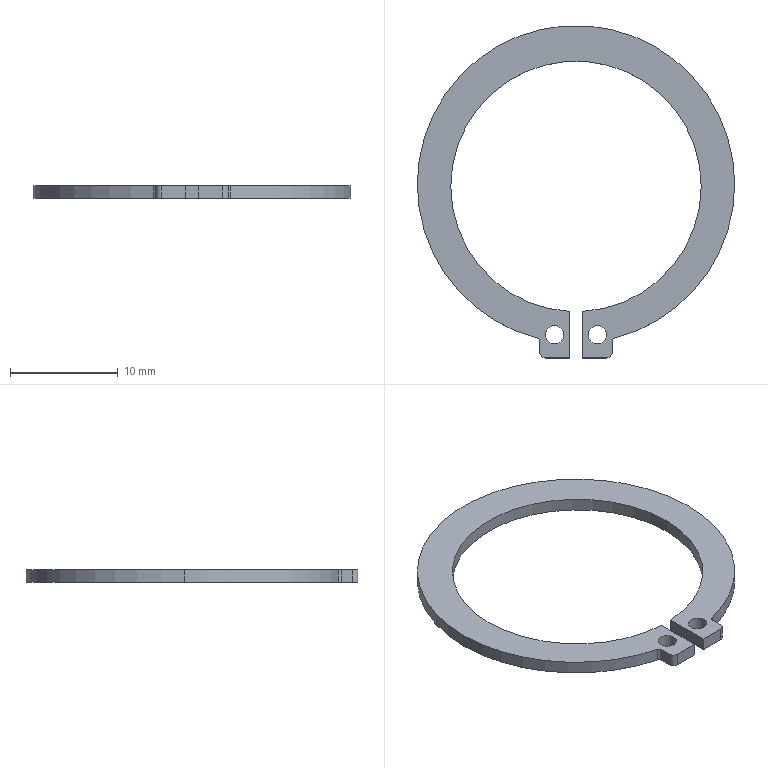Part | SolidWorks | features MBimport 1 | 1 solid | 22 faces | box 29.4 x 30.8 x 1.2 mm | volume 307.898 mm3 | cylinder 14 | plane 8 | commonest cylinder face diameters 1.7 x4 23.2 x3 29.4 x3 0.6 x2 1 x2
STEP:
#1=CARTESIAN_POINT('',(2.825,-13.75,0.));
#2=VERTEX_POINT('',#1);
#3=CARTESIAN_POINT('',(1.125,-13.75,0.));
#4=VERTEX_POINT('',#3);
#5=CARTESIAN_POINT('',(1.975,-13.75,0.));
#6=DIRECTION('',(0.,0.,1.));
#7=DIRECTION('',(1.,0.,0.));
#8=AXIS2_PLACEMENT_3D('',#5,#6,#7);
#9=CIRCLE('',#8,0.85);
#10=EDGE_CURVE('',#2,#4,#9,.T.);
#11=ORIENTED_EDGE('',*,*,#10,.F.);
#12=CARTESIAN_POINT('',(2.825,-13.75,1.2));
#13=VERTEX_POINT('',#12);
#14=CARTESIAN_POINT('',(2.825,-13.75,1.2));
#15=DIRECTION('',(0.,0.,1.));
#16=VECTOR('',#15,1000.);
#17=LINE('',#14,#16);
#18=EDGE_CURVE('',#2,#13,#17,.T.);
#19=ORIENTED_EDGE('',*,*,#18,.T.);
#20=CARTESIAN_POINT('',(1.125,-13.75,1.2));
#21=VERTEX_POINT('',#20);
#22=CARTESIAN_POINT('',(1.975,-13.75,1.2));
#23=DIRECTION('',(0.,0.,1.));
#24=DIRECTION('',(1.,0.,0.));
#25=AXIS2_PLACEMENT_3D('',#22,#23,#24);
#26=CIRCLE('',#25,0.85);
#27=EDGE_CURVE('',#13,#21,#26,.T.);
#28=ORIENTED_EDGE('',*,*,#27,.T.);
#29=CARTESIAN_POINT('',(1.125,-13.75,1.2));
#30=DIRECTION('',(0.,0.,1.));
#31=VECTOR('',#30,1000.);
#32=LINE('',#29,#31);
#33=EDGE_CURVE('',#4,#21,#32,.T.);
#34=ORIENTED_EDGE('',*,*,#33,.F.);
#35=EDGE_LOOP('',(#11,#19,#28,#34));
#36=FACE_OUTER_BOUND('',#35,.T.);
#37=CARTESIAN_POINT('',(1.975,-13.75,1.2));
#38=DIRECTION('',(0.,0.,1.));
#39=DIRECTION('',(-1.,0.,0.));
#40=AXIS2_PLACEMENT_3D('',#37,#38,#39);
#41=CYLINDRICAL_SURFACE('',#40,0.85);
#42=ADVANCED_FACE('',(#36),#41,.F.);
#43=CARTESIAN_POINT('',(3.577,-14.058,0.));
#44=VERTEX_POINT('',#43);
#45=CARTESIAN_POINT('',(14.7,0.2,0.));
#46=VERTEX_POINT('',#45);
#47=CARTESIAN_POINT('',(0.,0.2,0.));
#48=DIRECTION('',(0.,0.,1.));
#49=DIRECTION('',(1.,0.,0.));
#50=AXIS2_PLACEMENT_3D('',#47,#48,#49);
#51=CIRCLE('',#50,14.7);
#52=EDGE_CURVE('',#44,#46,#51,.T.);
#53=ORIENTED_EDGE('',*,*,#52,.T.);
#54=CARTESIAN_POINT('',(14.7,0.2,1.2));
#55=VERTEX_POINT('',#54);
#56=CARTESIAN_POINT('',(14.7,0.2,1.2));
#57=DIRECTION('',(0.,0.,1.));
#58=VECTOR('',#57,1000.);
#59=LINE('',#56,#58);
#60=EDGE_CURVE('',#46,#55,#59,.T.);
#61=ORIENTED_EDGE('',*,*,#60,.T.);
#62=CARTESIAN_POINT('',(3.577,-14.058,1.2));
#63=VERTEX_POINT('',#62);
#64=CARTESIAN_POINT('',(0.,0.2,1.2));
#65=DIRECTION('',(0.,0.,1.));
#66=DIRECTION('',(1.,0.,0.));
#67=AXIS2_PLACEMENT_3D('',#64,#65,#66);
#68=CIRCLE('',#67,14.7);
#69=EDGE_CURVE('',#63,#55,#68,.T.);
#70=ORIENTED_EDGE('',*,*,#69,.F.);
#71=CARTESIAN_POINT('',(3.577,-14.058,1.2));
#72=DIRECTION('',(0.,0.,-1.));
#73=VECTOR('',#72,1000.);
#74=LINE('',#71,#73);
#75=EDGE_CURVE('',#63,#44,#74,.T.);
#76=ORIENTED_EDGE('',*,*,#75,.T.);
#77=EDGE_LOOP('',(#53,#61,#70,#76));
#78=FACE_OUTER_BOUND('',#77,.T.);
#79=CARTESIAN_POINT('',(0.,0.2,1.2));
#80=DIRECTION('',(0.,0.,1.));
#81=DIRECTION('',(-1.,0.,0.));
#82=AXIS2_PLACEMENT_3D('',#79,#80,#81);
#83=CYLINDRICAL_SURFACE('',#82,14.7);
#84=ADVANCED_FACE('',(#78),#83,.T.);
#85=ORIENTED_EDGE('',*,*,#60,.F.);
#86=CARTESIAN_POINT('',(-14.7,0.2,0.));
#87=VERTEX_POINT('',#86);
#88=CARTESIAN_POINT('',(0.,0.2,0.));
#89=DIRECTION('',(0.,0.,1.));
#90=DIRECTION('',(1.,0.,0.));
#91=AXIS2_PLACEMENT_3D('',#88,#89,#90);
#92=CIRCLE('',#91,14.7);
#93=EDGE_CURVE('',#46,#87,#92,.T.);
#94=ORIENTED_EDGE('',*,*,#93,.T.);
#95=CARTESIAN_POINT('',(-14.7,0.2,1.2));
#96=VERTEX_POINT('',#95);
#97=CARTESIAN_POINT('',(-14.7,0.2,1.2));
#98=DIRECTION('',(0.,0.,1.));
#99=VECTOR('',#98,1000.);
#100=LINE('',#97,#99);
#101=EDGE_CURVE('',#87,#96,#100,.T.);
#102=ORIENTED_EDGE('',*,*,#101,.T.);
#103=CARTESIAN_POINT('',(0.,0.2,1.2));
#104=DIRECTION('',(0.,0.,1.));
#105=DIRECTION('',(1.,0.,0.));
#106=AXIS2_PLACEMENT_3D('',#103,#104,#105);
#107=CIRCLE('',#106,14.7);
#108=EDGE_CURVE('',#55,#96,#107,.T.);
#109=ORIENTED_EDGE('',*,*,#108,.F.);
#110=EDGE_LOOP('',(#85,#94,#102,#109));
#111=FACE_OUTER_BOUND('',#110,.T.);
#112=CARTESIAN_POINT('',(0.,0.2,1.2));
#113=DIRECTION('',(0.,0.,1.));
#114=DIRECTION('',(-1.,0.,0.));
#115=AXIS2_PLACEMENT_3D('',#112,#113,#114);
#116=CYLINDRICAL_SURFACE('',#115,14.7);
#117=ADVANCED_FACE('',(#111),#116,.T.);
#118=CARTESIAN_POINT('',(-1.125,-13.75,0.));
#119=VERTEX_POINT('',#118);
#120=CARTESIAN_POINT('',(-2.825,-13.75,0.));
#121=VERTEX_POINT('',#120);
#122=CARTESIAN_POINT('',(-1.975,-13.75,0.));
#123=DIRECTION('',(0.,0.,1.));
#124=DIRECTION('',(1.,0.,0.));
#125=AXIS2_PLACEMENT_3D('',#122,#123,#124);
#126=CIRCLE('',#125,0.85);
#127=EDGE_CURVE('',#119,#121,#126,.T.);
#128=ORIENTED_EDGE('',*,*,#127,.F.);
#129=CARTESIAN_POINT('',(-1.125,-13.75,1.2));
#130=VERTEX_POINT('',#129);
#131=CARTESIAN_POINT('',(-1.125,-13.75,1.2));
#132=DIRECTION('',(0.,0.,1.));
#133=VECTOR('',#132,1000.);
#134=LINE('',#131,#133);
#135=EDGE_CURVE('',#119,#130,#134,.T.);
#136=ORIENTED_EDGE('',*,*,#135,.T.);
#137=CARTESIAN_POINT('',(-2.825,-13.75,1.2));
#138=VERTEX_POINT('',#137);
#139=CARTESIAN_POINT('',(-1.975,-13.75,1.2));
#140=DIRECTION('',(0.,0.,1.));
#141=DIRECTION('',(1.,0.,0.));
#142=AXIS2_PLACEMENT_3D('',#139,#140,#141);
#143=CIRCLE('',#142,0.85);
#144=EDGE_CURVE('',#130,#138,#143,.T.);
#145=ORIENTED_EDGE('',*,*,#144,.T.);
#146=CARTESIAN_POINT('',(-2.825,-13.75,1.2));
#147=DIRECTION('',(0.,0.,1.));
#148=VECTOR('',#147,1000.);
#149=LINE('',#146,#148);
#150=EDGE_CURVE('',#121,#138,#149,.T.);
#151=ORIENTED_EDGE('',*,*,#150,.F.);
#152=EDGE_LOOP('',(#128,#136,#145,#151));
#153=FACE_OUTER_BOUND('',#152,.T.);
#154=CARTESIAN_POINT('',(-1.975,-13.75,1.2));
#155=DIRECTION('',(0.,0.,1.));
#156=DIRECTION('',(-1.,0.,0.));
#157=AXIS2_PLACEMENT_3D('',#154,#155,#156);
#158=CYLINDRICAL_SURFACE('',#157,0.85);
#159=ADVANCED_FACE('',(#153),#158,.F.);
#160=CARTESIAN_POINT('',(11.6,0.,0.));
#161=VERTEX_POINT('',#160);
#162=CARTESIAN_POINT('',(-11.6,0.,0.));
#163=VERTEX_POINT('',#162);
#164=CARTESIAN_POINT('',(0.,0.,0.));
#165=DIRECTION('',(0.,0.,1.));
#166=DIRECTION('',(1.,0.,0.));
#167=AXIS2_PLACEMENT_3D('',#164,#165,#166);
#168=CIRCLE('',#167,11.6);
#169=EDGE_CURVE('',#161,#163,#168,.T.);
#170=ORIENTED_EDGE('',*,*,#169,.F.);
#171=CARTESIAN_POINT('',(11.6,0.,1.2));
#172=VERTEX_POINT('',#171);
#173=CARTESIAN_POINT('',(11.6,0.,1.2));
#174=DIRECTION('',(0.,0.,1.));
#175=VECTOR('',#174,1000.);
#176=LINE('',#173,#175);
#177=EDGE_CURVE('',#161,#172,#176,.T.);
#178=ORIENTED_EDGE('',*,*,#177,.T.);
#179=CARTESIAN_POINT('',(-11.6,0.,1.2));
#180=VERTEX_POINT('',#179);
#181=CARTESIAN_POINT('',(0.,0.,1.2));
#182=DIRECTION('',(0.,0.,1.));
#183=DIRECTION('',(1.,0.,0.));
#184=AXIS2_PLACEMENT_3D('',#181,#182,#183);
#185=CIRCLE('',#184,11.6);
#186=EDGE_CURVE('',#172,#180,#185,.T.);
#187=ORIENTED_EDGE('',*,*,#186,.T.);
#188=CARTESIAN_POINT('',(-11.6,0.,1.2));
#189=DIRECTION('',(0.,0.,1.));
#190=VECTOR('',#189,1000.);
#191=LINE('',#188,#190);
#192=EDGE_CURVE('',#163,#180,#191,.T.);
#193=ORIENTED_EDGE('',*,*,#192,.F.);
#194=EDGE_LOOP('',(#170,#178,#187,#193));
#195=FACE_OUTER_BOUND('',#194,.T.);
#196=CARTESIAN_POINT('',(0.,0.,1.2));
#197=DIRECTION('',(0.,0.,1.));
#198=DIRECTION('',(-1.,0.,0.));
#199=AXIS2_PLACEMENT_3D('',#196,#197,#198);
#200=CYLINDRICAL_SURFACE('',#199,11.6);
#201=ADVANCED_FACE('',(#195),#200,.F.);
#202=CARTESIAN_POINT('',(-0.6,-11.584,0.));
#203=VERTEX_POINT('',#202);
#204=CARTESIAN_POINT('',(0.,0.,0.));
#205=DIRECTION('',(0.,0.,1.));
#206=DIRECTION('',(1.,0.,0.));
#207=AXIS2_PLACEMENT_3D('',#204,#205,#206);
#208=CIRCLE('',#207,11.6);
#209=EDGE_CURVE('',#163,#203,#208,.T.);
#210=ORIENTED_EDGE('',*,*,#209,.F.);
#211=ORIENTED_EDGE('',*,*,#192,.T.);
#212=CARTESIAN_POINT('',(-0.6,-11.584,1.2));
#213=VERTEX_POINT('',#212);
#214=CARTESIAN_POINT('',(0.,0.,1.2));
#215=DIRECTION('',(0.,0.,1.));
#216=DIRECTION('',(1.,0.,0.));
#217=AXIS2_PLACEMENT_3D('',#214,#215,#216);
#218=CIRCLE('',#217,11.6);
#219=EDGE_CURVE('',#180,#213,#218,.T.);
#220=ORIENTED_EDGE('',*,*,#219,.T.);
#221=CARTESIAN_POINT('',(-0.6,-11.584,1.2));
#222=DIRECTION('',(0.,0.,-1.));
#223=VECTOR('',#222,1000.);
#224=LINE('',#221,#223);
#225=EDGE_CURVE('',#213,#203,#224,.T.);
#226=ORIENTED_EDGE('',*,*,#225,.T.);
#227=EDGE_LOOP('',(#210,#211,#220,#226));
#228=FACE_OUTER_BOUND('',#227,.T.);
#229=CARTESIAN_POINT('',(0.,0.,1.2));
#230=DIRECTION('',(0.,0.,1.));
#231=DIRECTION('',(-1.,0.,0.));
#232=AXIS2_PLACEMENT_3D('',#229,#230,#231);
#233=CYLINDRICAL_SURFACE('',#232,11.6);
#234=ADVANCED_FACE('',(#228),#233,.F.);
#235=CARTESIAN_POINT('',(3.35,-14.349,1.2));
#236=VERTEX_POINT('',#235);
#237=CARTESIAN_POINT('',(3.65,-14.349,1.2));
#238=DIRECTION('',(0.,0.,1.));
#239=DIRECTION('',(1.,0.,0.));
#240=AXIS2_PLACEMENT_3D('',#237,#238,#239);
#241=CIRCLE('',#240,0.3);
#242=EDGE_CURVE('',#63,#236,#241,.T.);
#243=ORIENTED_EDGE('',*,*,#242,.F.);
#244=ORIENTED_EDGE('',*,*,#69,.T.);
#245=ORIENTED_EDGE('',*,*,#108,.T.);
#246=CARTESIAN_POINT('',(-3.577,-14.058,1.2));
#247=VERTEX_POINT('',#246);
#248=CARTESIAN_POINT('',(0.,0.2,1.2));
#249=DIRECTION('',(0.,0.,1.));
#250=DIRECTION('',(1.,0.,0.));
#251=AXIS2_PLACEMENT_3D('',#248,#249,#250);
#252=CIRCLE('',#251,14.7);
#253=EDGE_CURVE('',#96,#247,#252,.T.);
#254=ORIENTED_EDGE('',*,*,#253,.T.);
#255=CARTESIAN_POINT('',(-3.35,-14.349,1.2));
#256=VERTEX_POINT('',#255);
#257=CARTESIAN_POINT('',(-3.65,-14.349,1.2));
#258=DIRECTION('',(0.,0.,1.));
#259=DIRECTION('',(1.,0.,0.));
#260=AXIS2_PLACEMENT_3D('',#257,#258,#259);
#261=CIRCLE('',#260,0.3);
#262=EDGE_CURVE('',#256,#247,#261,.T.);
#263=ORIENTED_EDGE('',*,*,#262,.F.);
#264=CARTESIAN_POINT('',(-3.35,-15.4,1.2));
#265=VERTEX_POINT('',#264);
#266=CARTESIAN_POINT('',(-3.35,-14.349,1.2));
#267=DIRECTION('',(0.,-1.,0.));
#268=VECTOR('',#267,1000.);
#269=LINE('',#266,#268);
#270=EDGE_CURVE('',#256,#265,#269,.T.);
#271=ORIENTED_EDGE('',*,*,#270,.T.);
#272=CARTESIAN_POINT('',(-2.85,-15.9,1.2));
#273=VERTEX_POINT('',#272);
#274=CARTESIAN_POINT('',(-2.85,-15.4,1.2));
#275=DIRECTION('',(0.,0.,1.));
#276=DIRECTION('',(1.,0.,0.));
#277=AXIS2_PLACEMENT_3D('',#274,#275,#276);
#278=CIRCLE('',#277,0.5);
#279=EDGE_CURVE('',#265,#273,#278,.T.);
#280=ORIENTED_EDGE('',*,*,#279,.T.);
#281=CARTESIAN_POINT('',(-0.6,-15.9,1.2));
#282=VERTEX_POINT('',#281);
#283=CARTESIAN_POINT('',(-2.85,-15.9,1.2));
#284=DIRECTION('',(1.,0.,0.));
#285=VECTOR('',#284,1000.);
#286=LINE('',#283,#285);
#287=EDGE_CURVE('',#273,#282,#286,.T.);
#288=ORIENTED_EDGE('',*,*,#287,.T.);
#289=CARTESIAN_POINT('',(-0.6,-15.9,1.2));
#290=DIRECTION('',(0.,1.,0.));
#291=VECTOR('',#290,1000.);
#292=LINE('',#289,#291);
#293=EDGE_CURVE('',#282,#213,#292,.T.);
#294=ORIENTED_EDGE('',*,*,#293,.T.);
#295=ORIENTED_EDGE('',*,*,#219,.F.);
#296=ORIENTED_EDGE('',*,*,#186,.F.);
#297=CARTESIAN_POINT('',(0.6,-11.584,1.2));
#298=VERTEX_POINT('',#297);
#299=CARTESIAN_POINT('',(0.,0.,1.2));
#300=DIRECTION('',(0.,0.,1.));
#301=DIRECTION('',(1.,0.,0.));
#302=AXIS2_PLACEMENT_3D('',#299,#300,#301);
#303=CIRCLE('',#302,11.6);
#304=EDGE_CURVE('',#298,#172,#303,.T.);
#305=ORIENTED_EDGE('',*,*,#304,.F.);
#306=CARTESIAN_POINT('',(0.6,-15.9,1.2));
#307=VERTEX_POINT('',#306);
#308=CARTESIAN_POINT('',(0.6,-11.584,1.2));
#309=DIRECTION('',(0.,-1.,0.));
#310=VECTOR('',#309,1000.);
#311=LINE('',#308,#310);
#312=EDGE_CURVE('',#298,#307,#311,.T.);
#313=ORIENTED_EDGE('',*,*,#312,.T.);
#314=CARTESIAN_POINT('',(2.85,-15.9,1.2));
#315=VERTEX_POINT('',#314);
#316=CARTESIAN_POINT('',(0.6,-15.9,1.2));
#317=DIRECTION('',(1.,0.,0.));
#318=VECTOR('',#317,1000.);
#319=LINE('',#316,#318);
#320=EDGE_CURVE('',#307,#315,#319,.T.);
#321=ORIENTED_EDGE('',*,*,#320,.T.);
#322=CARTESIAN_POINT('',(3.35,-15.4,1.2));
#323=VERTEX_POINT('',#322);
#324=CARTESIAN_POINT('',(2.85,-15.4,1.2));
#325=DIRECTION('',(0.,0.,1.));
#326=DIRECTION('',(1.,0.,0.));
#327=AXIS2_PLACEMENT_3D('',#324,#325,#326);
#328=CIRCLE('',#327,0.5);
#329=EDGE_CURVE('',#315,#323,#328,.T.);
#330=ORIENTED_EDGE('',*,*,#329,.T.);
#331=CARTESIAN_POINT('',(3.35,-15.4,1.2));
#332=DIRECTION('',(0.,1.,0.));
#333=VECTOR('',#332,1000.);
#334=LINE('',#331,#333);
#335=EDGE_CURVE('',#323,#236,#334,.T.);
#336=ORIENTED_EDGE('',*,*,#335,.T.);
#337=EDGE_LOOP('',(#243,#244,#245,#254,#263,#271,#280,#288,#294,#295,#296,#305,#313,#321,#330,#336));
#338=FACE_OUTER_BOUND('',#337,.T.);
#339=CARTESIAN_POINT('',(-1.975,-13.75,1.2));
#340=DIRECTION('',(0.,0.,1.));
#341=DIRECTION('',(1.,0.,0.));
#342=AXIS2_PLACEMENT_3D('',#339,#340,#341);
#343=CIRCLE('',#342,0.85);
#344=EDGE_CURVE('',#138,#130,#343,.T.);
#345=ORIENTED_EDGE('',*,*,#344,.F.);
#346=ORIENTED_EDGE('',*,*,#144,.F.);
#347=EDGE_LOOP('',(#345,#346));
#348=FACE_BOUND('',#347,.T.);
#349=CARTESIAN_POINT('',(1.975,-13.75,1.2));
#350=DIRECTION('',(0.,0.,1.));
#351=DIRECTION('',(1.,0.,0.));
#352=AXIS2_PLACEMENT_3D('',#349,#350,#351);
#353=CIRCLE('',#352,0.85);
#354=EDGE_CURVE('',#21,#13,#353,.T.);
#355=ORIENTED_EDGE('',*,*,#354,.F.);
#356=ORIENTED_EDGE('',*,*,#27,.F.);
#357=EDGE_LOOP('',(#355,#356));
#358=FACE_BOUND('',#357,.T.);
#359=CARTESIAN_POINT('',(3.65,-14.349,1.2));
#360=DIRECTION('',(0.,0.,1.));
#361=DIRECTION('',(1.,0.,0.));
#362=AXIS2_PLACEMENT_3D('',#359,#360,#361);
#363=PLANE('',#362);
#364=ADVANCED_FACE('',(#338,#348,#358),#363,.T.);
#365=CARTESIAN_POINT('',(3.35,-14.349,0.));
#366=VERTEX_POINT('',#365);
#367=CARTESIAN_POINT('',(3.65,-14.349,0.));
#368=DIRECTION('',(0.,0.,1.));
#369=DIRECTION('',(1.,0.,0.));
#370=AXIS2_PLACEMENT_3D('',#367,#368,#369);
#371=CIRCLE('',#370,0.3);
#372=EDGE_CURVE('',#44,#366,#371,.T.);
#373=ORIENTED_EDGE('',*,*,#372,.F.);
#374=ORIENTED_EDGE('',*,*,#75,.F.);
#375=ORIENTED_EDGE('',*,*,#242,.T.);
#376=CARTESIAN_POINT('',(3.35,-14.349,1.2));
#377=DIRECTION('',(0.,0.,-1.));
#378=VECTOR('',#377,1000.);
#379=LINE('',#376,#378);
#380=EDGE_CURVE('',#236,#366,#379,.T.);
#381=ORIENTED_EDGE('',*,*,#380,.T.);
#382=EDGE_LOOP('',(#373,#374,#375,#381));
#383=FACE_OUTER_BOUND('',#382,.T.);
#384=CARTESIAN_POINT('',(3.65,-14.349,1.2));
#385=DIRECTION('',(0.,0.,1.));
#386=DIRECTION('',(-1.,0.,0.));
#387=AXIS2_PLACEMENT_3D('',#384,#385,#386);
#388=CYLINDRICAL_SURFACE('',#387,0.3);
#389=ADVANCED_FACE('',(#383),#388,.F.);
#390=CARTESIAN_POINT('',(-3.35,-14.349,0.));
#391=VERTEX_POINT('',#390);
#392=CARTESIAN_POINT('',(-3.577,-14.058,0.));
#393=VERTEX_POINT('',#392);
#394=CARTESIAN_POINT('',(-3.65,-14.349,0.));
#395=DIRECTION('',(0.,0.,1.));
#396=DIRECTION('',(1.,0.,0.));
#397=AXIS2_PLACEMENT_3D('',#394,#395,#396);
#398=CIRCLE('',#397,0.3);
#399=EDGE_CURVE('',#391,#393,#398,.T.);
#400=ORIENTED_EDGE('',*,*,#399,.F.);
#401=CARTESIAN_POINT('',(-3.35,-14.349,1.2));
#402=DIRECTION('',(0.,0.,-1.));
#403=VECTOR('',#402,1000.);
#404=LINE('',#401,#403);
#405=EDGE_CURVE('',#256,#391,#404,.T.);
#406=ORIENTED_EDGE('',*,*,#405,.F.);
#407=ORIENTED_EDGE('',*,*,#262,.T.);
#408=CARTESIAN_POINT('',(-3.577,-14.058,1.2));
#409=DIRECTION('',(0.,0.,-1.));
#410=VECTOR('',#409,1000.);
#411=LINE('',#408,#410);
#412=EDGE_CURVE('',#247,#393,#411,.T.);
#413=ORIENTED_EDGE('',*,*,#412,.T.);
#414=EDGE_LOOP('',(#400,#406,#407,#413));
#415=FACE_OUTER_BOUND('',#414,.T.);
#416=CARTESIAN_POINT('',(-3.65,-14.349,1.2));
#417=DIRECTION('',(0.,0.,1.));
#418=DIRECTION('',(-1.,0.,0.));
#419=AXIS2_PLACEMENT_3D('',#416,#417,#418);
#420=CYLINDRICAL_SURFACE('',#419,0.3);
#421=ADVANCED_FACE('',(#415),#420,.F.);
#422=CARTESIAN_POINT('',(-3.35,-15.4,0.));
#423=VERTEX_POINT('',#422);
#424=CARTESIAN_POINT('',(-3.35,-14.349,0.));
#425=DIRECTION('',(0.,-1.,0.));
#426=VECTOR('',#425,1000.);
#427=LINE('',#424,#426);
#428=EDGE_CURVE('',#391,#423,#427,.T.);
#429=ORIENTED_EDGE('',*,*,#428,.T.);
#430=CARTESIAN_POINT('',(-3.35,-15.4,1.2));
#431=DIRECTION('',(0.,0.,-1.));
#432=VECTOR('',#431,1000.);
#433=LINE('',#430,#432);
#434=EDGE_CURVE('',#265,#423,#433,.T.);
#435=ORIENTED_EDGE('',*,*,#434,.F.);
#436=ORIENTED_EDGE('',*,*,#270,.F.);
#437=ORIENTED_EDGE('',*,*,#405,.T.);
#438=EDGE_LOOP('',(#429,#435,#436,#437));
#439=FACE_OUTER_BOUND('',#438,.T.);
#440=CARTESIAN_POINT('',(-3.35,-14.349,1.2));
#441=DIRECTION('',(1.,0.,0.));
#442=DIRECTION('',(0.,1.,0.));
#443=AXIS2_PLACEMENT_3D('',#440,#441,#442);
#444=PLANE('',#443);
#445=ADVANCED_FACE('',(#439),#444,.F.);
#446=CARTESIAN_POINT('',(3.35,-15.4,0.));
#447=VERTEX_POINT('',#446);
#448=CARTESIAN_POINT('',(3.35,-15.4,0.));
#449=DIRECTION('',(0.,1.,0.));
#450=VECTOR('',#449,1000.);
#451=LINE('',#448,#450);
#452=EDGE_CURVE('',#447,#366,#451,.T.);
#453=ORIENTED_EDGE('',*,*,#452,.T.);
#454=ORIENTED_EDGE('',*,*,#380,.F.);
#455=ORIENTED_EDGE('',*,*,#335,.F.);
#456=CARTESIAN_POINT('',(3.35,-15.4,1.2));
#457=DIRECTION('',(0.,0.,-1.));
#458=VECTOR('',#457,1000.);
#459=LINE('',#456,#458);
#460=EDGE_CURVE('',#323,#447,#459,.T.);
#461=ORIENTED_EDGE('',*,*,#460,.T.);
#462=EDGE_LOOP('',(#453,#454,#455,#461));
#463=FACE_OUTER_BOUND('',#462,.T.);
#464=CARTESIAN_POINT('',(3.35,-15.4,1.2));
#465=DIRECTION('',(-1.,0.,0.));
#466=DIRECTION('',(0.,0.,1.));
#467=AXIS2_PLACEMENT_3D('',#464,#465,#466);
#468=PLANE('',#467);
#469=ADVANCED_FACE('',(#463),#468,.F.);
#470=CARTESIAN_POINT('',(2.85,-15.9,0.));
#471=VERTEX_POINT('',#470);
#472=CARTESIAN_POINT('',(2.85,-15.4,0.));
#473=DIRECTION('',(0.,0.,1.));
#474=DIRECTION('',(1.,0.,0.));
#475=AXIS2_PLACEMENT_3D('',#472,#473,#474);
#476=CIRCLE('',#475,0.5);
#477=EDGE_CURVE('',#471,#447,#476,.T.);
#478=ORIENTED_EDGE('',*,*,#477,.T.);
#479=ORIENTED_EDGE('',*,*,#460,.F.);
#480=ORIENTED_EDGE('',*,*,#329,.F.);
#481=CARTESIAN_POINT('',(2.85,-15.9,1.2));
#482=DIRECTION('',(0.,0.,-1.));
#483=VECTOR('',#482,1000.);
#484=LINE('',#481,#483);
#485=EDGE_CURVE('',#315,#471,#484,.T.);
#486=ORIENTED_EDGE('',*,*,#485,.T.);
#487=EDGE_LOOP('',(#478,#479,#480,#486));
#488=FACE_OUTER_BOUND('',#487,.T.);
#489=CARTESIAN_POINT('',(2.85,-15.4,1.2));
#490=DIRECTION('',(0.,0.,1.));
#491=DIRECTION('',(-1.,0.,0.));
#492=AXIS2_PLACEMENT_3D('',#489,#490,#491);
#493=CYLINDRICAL_SURFACE('',#492,0.5);
#494=ADVANCED_FACE('',(#488),#493,.T.);
#495=ORIENTED_EDGE('',*,*,#372,.T.);
#496=ORIENTED_EDGE('',*,*,#452,.F.);
#497=ORIENTED_EDGE('',*,*,#477,.F.);
#498=CARTESIAN_POINT('',(0.6,-15.9,0.));
#499=VERTEX_POINT('',#498);
#500=CARTESIAN_POINT('',(0.6,-15.9,0.));
#501=DIRECTION('',(1.,0.,0.));
#502=VECTOR('',#501,1000.);
#503=LINE('',#500,#502);
#504=EDGE_CURVE('',#499,#471,#503,.T.);
#505=ORIENTED_EDGE('',*,*,#504,.F.);
#506=CARTESIAN_POINT('',(0.6,-11.584,0.));
#507=VERTEX_POINT('',#506);
#508=CARTESIAN_POINT('',(0.6,-11.584,0.));
#509=DIRECTION('',(0.,-1.,0.));
#510=VECTOR('',#509,1000.);
#511=LINE('',#508,#510);
#512=EDGE_CURVE('',#507,#499,#511,.T.);
#513=ORIENTED_EDGE('',*,*,#512,.F.);
#514=CARTESIAN_POINT('',(0.,0.,0.));
#515=DIRECTION('',(0.,0.,1.));
#516=DIRECTION('',(1.,0.,0.));
#517=AXIS2_PLACEMENT_3D('',#514,#515,#516);
#518=CIRCLE('',#517,11.6);
#519=EDGE_CURVE('',#507,#161,#518,.T.);
#520=ORIENTED_EDGE('',*,*,#519,.T.);
#521=ORIENTED_EDGE('',*,*,#169,.T.);
#522=ORIENTED_EDGE('',*,*,#209,.T.);
#523=CARTESIAN_POINT('',(-0.6,-15.9,0.));
#524=VERTEX_POINT('',#523);
#525=CARTESIAN_POINT('',(-0.6,-15.9,0.));
#526=DIRECTION('',(0.,1.,0.));
#527=VECTOR('',#526,1000.);
#528=LINE('',#525,#527);
#529=EDGE_CURVE('',#524,#203,#528,.T.);
#530=ORIENTED_EDGE('',*,*,#529,.F.);
#531=CARTESIAN_POINT('',(-2.85,-15.9,0.));
#532=VERTEX_POINT('',#531);
#533=CARTESIAN_POINT('',(-2.85,-15.9,0.));
#534=DIRECTION('',(1.,0.,0.));
#535=VECTOR('',#534,1000.);
#536=LINE('',#533,#535);
#537=EDGE_CURVE('',#532,#524,#536,.T.);
#538=ORIENTED_EDGE('',*,*,#537,.F.);
#539=CARTESIAN_POINT('',(-2.85,-15.4,0.));
#540=DIRECTION('',(0.,0.,1.));
#541=DIRECTION('',(1.,0.,0.));
#542=AXIS2_PLACEMENT_3D('',#539,#540,#541);
#543=CIRCLE('',#542,0.5);
#544=EDGE_CURVE('',#423,#532,#543,.T.);
#545=ORIENTED_EDGE('',*,*,#544,.F.);
#546=ORIENTED_EDGE('',*,*,#428,.F.);
#547=ORIENTED_EDGE('',*,*,#399,.T.);
#548=CARTESIAN_POINT('',(0.,0.2,0.));
#549=DIRECTION('',(0.,0.,1.));
#550=DIRECTION('',(1.,0.,0.));
#551=AXIS2_PLACEMENT_3D('',#548,#549,#550);
#552=CIRCLE('',#551,14.7);
#553=EDGE_CURVE('',#87,#393,#552,.T.);
#554=ORIENTED_EDGE('',*,*,#553,.F.);
#555=ORIENTED_EDGE('',*,*,#93,.F.);
#556=ORIENTED_EDGE('',*,*,#52,.F.);
#557=EDGE_LOOP('',(#495,#496,#497,#505,#513,#520,#521,#522,#530,#538,#545,#546,#547,#554,#555,#556));
#558=FACE_OUTER_BOUND('',#557,.T.);
#559=CARTESIAN_POINT('',(-1.975,-13.75,0.));
#560=DIRECTION('',(0.,0.,1.));
#561=DIRECTION('',(1.,0.,0.));
#562=AXIS2_PLACEMENT_3D('',#559,#560,#561);
#563=CIRCLE('',#562,0.85);
#564=EDGE_CURVE('',#121,#119,#563,.T.);
#565=ORIENTED_EDGE('',*,*,#564,.T.);
#566=ORIENTED_EDGE('',*,*,#127,.T.);
#567=EDGE_LOOP('',(#565,#566));
#568=FACE_BOUND('',#567,.T.);
#569=CARTESIAN_POINT('',(1.975,-13.75,0.));
#570=DIRECTION('',(0.,0.,1.));
#571=DIRECTION('',(1.,0.,0.));
#572=AXIS2_PLACEMENT_3D('',#569,#570,#571);
#573=CIRCLE('',#572,0.85);
#574=EDGE_CURVE('',#4,#2,#573,.T.);
#575=ORIENTED_EDGE('',*,*,#574,.T.);
#576=ORIENTED_EDGE('',*,*,#10,.T.);
#577=EDGE_LOOP('',(#575,#576));
#578=FACE_BOUND('',#577,.T.);
#579=CARTESIAN_POINT('',(3.65,-14.349,0.));
#580=DIRECTION('',(0.,0.,1.));
#581=DIRECTION('',(1.,0.,0.));
#582=AXIS2_PLACEMENT_3D('',#579,#580,#581);
#583=PLANE('',#582);
#584=ADVANCED_FACE('',(#558,#568,#578),#583,.F.);
#585=ORIENTED_EDGE('',*,*,#544,.T.);
#586=CARTESIAN_POINT('',(-2.85,-15.9,1.2));
#587=DIRECTION('',(0.,0.,-1.));
#588=VECTOR('',#587,1000.);
#589=LINE('',#586,#588);
#590=EDGE_CURVE('',#273,#532,#589,.T.);
#591=ORIENTED_EDGE('',*,*,#590,.F.);
#592=ORIENTED_EDGE('',*,*,#279,.F.);
#593=ORIENTED_EDGE('',*,*,#434,.T.);
#594=EDGE_LOOP('',(#585,#591,#592,#593));
#595=FACE_OUTER_BOUND('',#594,.T.);
#596=CARTESIAN_POINT('',(-2.85,-15.4,1.2));
#597=DIRECTION('',(0.,0.,1.));
#598=DIRECTION('',(-1.,0.,0.));
#599=AXIS2_PLACEMENT_3D('',#596,#597,#598);
#600=CYLINDRICAL_SURFACE('',#599,0.5);
#601=ADVANCED_FACE('',(#595),#600,.T.);
#602=ORIENTED_EDGE('',*,*,#537,.T.);
#603=CARTESIAN_POINT('',(-0.6,-15.9,1.2));
#604=DIRECTION('',(0.,0.,-1.));
#605=VECTOR('',#604,1000.);
#606=LINE('',#603,#605);
#607=EDGE_CURVE('',#282,#524,#606,.T.);
#608=ORIENTED_EDGE('',*,*,#607,.F.);
#609=ORIENTED_EDGE('',*,*,#287,.F.);
#610=ORIENTED_EDGE('',*,*,#590,.T.);
#611=EDGE_LOOP('',(#602,#608,#609,#610));
#612=FACE_OUTER_BOUND('',#611,.T.);
#613=CARTESIAN_POINT('',(-2.85,-15.9,1.2));
#614=DIRECTION('',(0.,1.,0.));
#615=DIRECTION('',(1.,0.,0.));
#616=AXIS2_PLACEMENT_3D('',#613,#614,#615);
#617=PLANE('',#616);
#618=ADVANCED_FACE('',(#612),#617,.F.);
#619=ORIENTED_EDGE('',*,*,#529,.T.);
#620=ORIENTED_EDGE('',*,*,#225,.F.);
#621=ORIENTED_EDGE('',*,*,#293,.F.);
#622=ORIENTED_EDGE('',*,*,#607,.T.);
#623=EDGE_LOOP('',(#619,#620,#621,#622));
#624=FACE_OUTER_BOUND('',#623,.T.);
#625=CARTESIAN_POINT('',(-0.6,-15.9,1.2));
#626=DIRECTION('',(-1.,0.,0.));
#627=DIRECTION('',(0.,1.,0.));
#628=AXIS2_PLACEMENT_3D('',#625,#626,#627);
#629=PLANE('',#628);
#630=ADVANCED_FACE('',(#624),#629,.F.);
#631=ORIENTED_EDGE('',*,*,#177,.F.);
#632=ORIENTED_EDGE('',*,*,#519,.F.);
#633=CARTESIAN_POINT('',(0.6,-11.584,1.2));
#634=DIRECTION('',(0.,0.,-1.));
#635=VECTOR('',#634,1000.);
#636=LINE('',#633,#635);
#637=EDGE_CURVE('',#298,#507,#636,.T.);
#638=ORIENTED_EDGE('',*,*,#637,.F.);
#639=ORIENTED_EDGE('',*,*,#304,.T.);
#640=EDGE_LOOP('',(#631,#632,#638,#639));
#641=FACE_OUTER_BOUND('',#640,.T.);
#642=CARTESIAN_POINT('',(0.,0.,1.2));
#643=DIRECTION('',(0.,0.,1.));
#644=DIRECTION('',(-1.,0.,0.));
#645=AXIS2_PLACEMENT_3D('',#642,#643,#644);
#646=CYLINDRICAL_SURFACE('',#645,11.6);
#647=ADVANCED_FACE('',(#641),#646,.F.);
#648=ORIENTED_EDGE('',*,*,#512,.T.);
#649=CARTESIAN_POINT('',(0.6,-15.9,1.2));
#650=DIRECTION('',(0.,0.,-1.));
#651=VECTOR('',#650,1000.);
#652=LINE('',#649,#651);
#653=EDGE_CURVE('',#307,#499,#652,.T.);
#654=ORIENTED_EDGE('',*,*,#653,.F.);
#655=ORIENTED_EDGE('',*,*,#312,.F.);
#656=ORIENTED_EDGE('',*,*,#637,.T.);
#657=EDGE_LOOP('',(#648,#654,#655,#656));
#658=FACE_OUTER_BOUND('',#657,.T.);
#659=CARTESIAN_POINT('',(0.6,-11.584,1.2));
#660=DIRECTION('',(1.,0.,0.));
#661=DIRECTION('',(0.,1.,0.));
#662=AXIS2_PLACEMENT_3D('',#659,#660,#661);
#663=PLANE('',#662);
#664=ADVANCED_FACE('',(#658),#663,.F.);
#665=ORIENTED_EDGE('',*,*,#504,.T.);
#666=ORIENTED_EDGE('',*,*,#485,.F.);
#667=ORIENTED_EDGE('',*,*,#320,.F.);
#668=ORIENTED_EDGE('',*,*,#653,.T.);
#669=EDGE_LOOP('',(#665,#666,#667,#668));
#670=FACE_OUTER_BOUND('',#669,.T.);
#671=CARTESIAN_POINT('',(0.6,-15.9,1.2));
#672=DIRECTION('',(0.,1.,0.));
#673=DIRECTION('',(1.,0.,0.));
#674=AXIS2_PLACEMENT_3D('',#671,#672,#673);
#675=PLANE('',#674);
#676=ADVANCED_FACE('',(#670),#675,.F.);
#677=ORIENTED_EDGE('',*,*,#135,.F.);
#678=ORIENTED_EDGE('',*,*,#564,.F.);
#679=ORIENTED_EDGE('',*,*,#150,.T.);
#680=ORIENTED_EDGE('',*,*,#344,.T.);
#681=EDGE_LOOP('',(#677,#678,#679,#680));
#682=FACE_OUTER_BOUND('',#681,.T.);
#683=CARTESIAN_POINT('',(-1.975,-13.75,1.2));
#684=DIRECTION('',(0.,0.,1.));
#685=DIRECTION('',(-1.,0.,0.));
#686=AXIS2_PLACEMENT_3D('',#683,#684,#685);
#687=CYLINDRICAL_SURFACE('',#686,0.85);
#688=ADVANCED_FACE('',(#682),#687,.F.);
#689=ORIENTED_EDGE('',*,*,#101,.F.);
#690=ORIENTED_EDGE('',*,*,#553,.T.);
#691=ORIENTED_EDGE('',*,*,#412,.F.);
#692=ORIENTED_EDGE('',*,*,#253,.F.);
#693=EDGE_LOOP('',(#689,#690,#691,#692));
#694=FACE_OUTER_BOUND('',#693,.T.);
#695=CARTESIAN_POINT('',(0.,0.2,1.2));
#696=DIRECTION('',(0.,0.,1.));
#697=DIRECTION('',(-1.,0.,0.));
#698=AXIS2_PLACEMENT_3D('',#695,#696,#697);
#699=CYLINDRICAL_SURFACE('',#698,14.7);
#700=ADVANCED_FACE('',(#694),#699,.T.);
#701=ORIENTED_EDGE('',*,*,#18,.F.);
#702=ORIENTED_EDGE('',*,*,#574,.F.);
#703=ORIENTED_EDGE('',*,*,#33,.T.);
#704=ORIENTED_EDGE('',*,*,#354,.T.);
#705=EDGE_LOOP('',(#701,#702,#703,#704));
#706=FACE_OUTER_BOUND('',#705,.T.);
#707=CARTESIAN_POINT('',(1.975,-13.75,1.2));
#708=DIRECTION('',(0.,0.,1.));
#709=DIRECTION('',(-1.,0.,0.));
#710=AXIS2_PLACEMENT_3D('',#707,#708,#709);
#711=CYLINDRICAL_SURFACE('',#710,0.85);
#712=ADVANCED_FACE('',(#706),#711,.F.);
#713=CLOSED_SHELL('',(#42,#84,#117,#159,#201,#234,#364,#389,#421,#445,#469,#494,#584,#601,#618,#630,#647,#664,#676,#688,#700,#712));
#714=MANIFOLD_SOLID_BREP('',#713);
#715=CARTESIAN_POINT('',(0.,0.,0.));
#716=DIRECTION('',(0.,0.,1.));
#717=DIRECTION('',(1.,0.,0.));
#718=AXIS2_PLACEMENT_3D('',#715,#716,#717);
#719=(LENGTH_UNIT()NAMED_UNIT(*)SI_UNIT(.MILLI.,.METRE.));
#720=UNCERTAINTY_MEASURE_WITH_UNIT(LENGTH_MEASURE(0.00001),#719,'','');
#721=(NAMED_UNIT(*)PLANE_ANGLE_UNIT()SI_UNIT($,.RADIAN.));
#722=(NAMED_UNIT(*)SI_UNIT($,.STERADIAN.)SOLID_ANGLE_UNIT());
#723=(GEOMETRIC_REPRESENTATION_CONTEXT(3)GLOBAL_UNCERTAINTY_ASSIGNED_CONTEXT((#720))GLOBAL_UNIT_ASSIGNED_CONTEXT((#719,#721,#722))REPRESENTATION_CONTEXT('',''));
#724=ADVANCED_BREP_SHAPE_REPRESENTATION('',(#714,#718),#723);